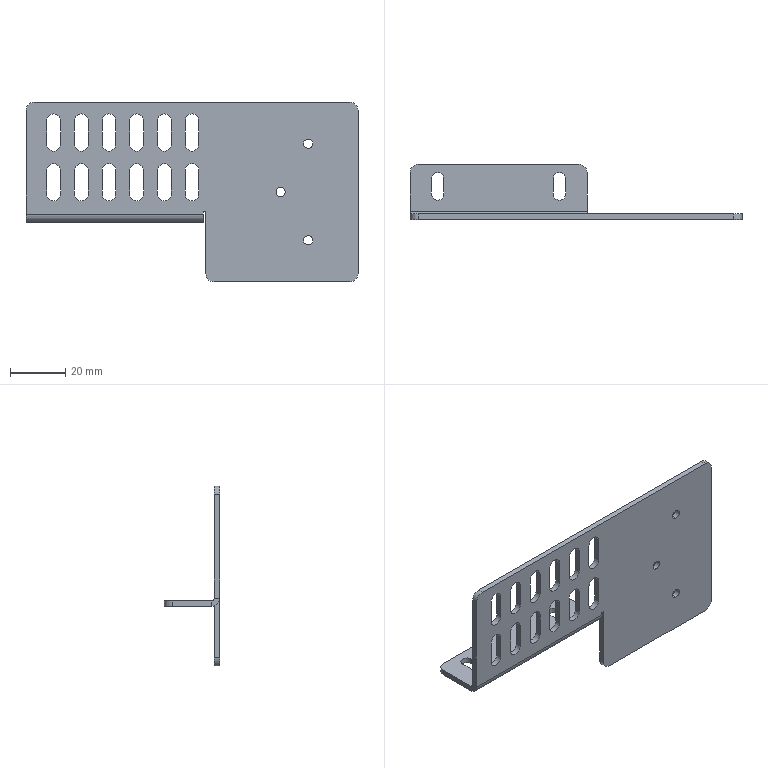Part | NX | features BREP 1 | 1 solid | 98 faces | box 120 x 20 x 65 mm | volume 13263 mm3 | cylinder 54 | plane 44 | commonest cylinder face diameters 5 x36 6 x7 3.3 x6 4.5 x4 2 x1